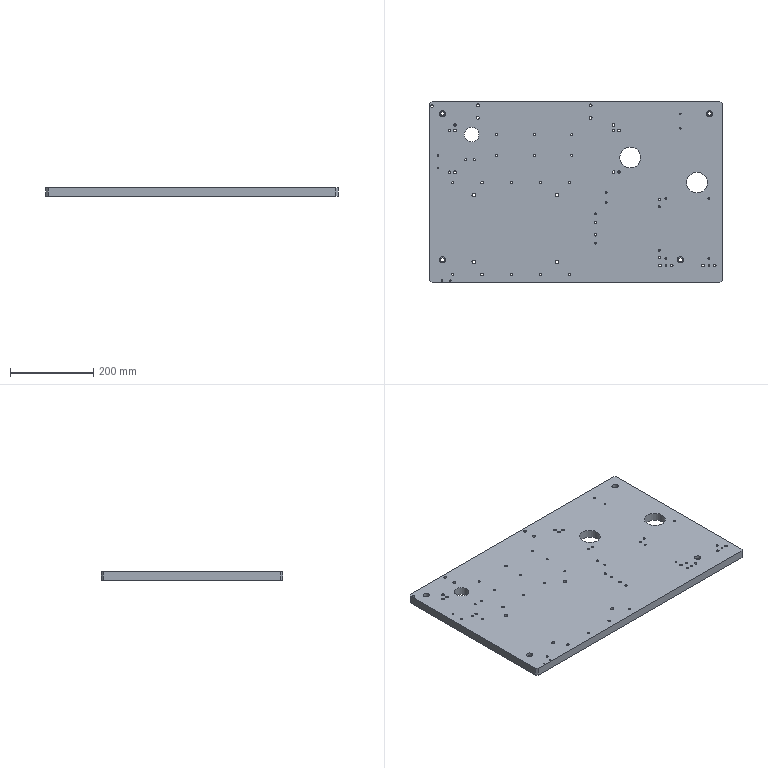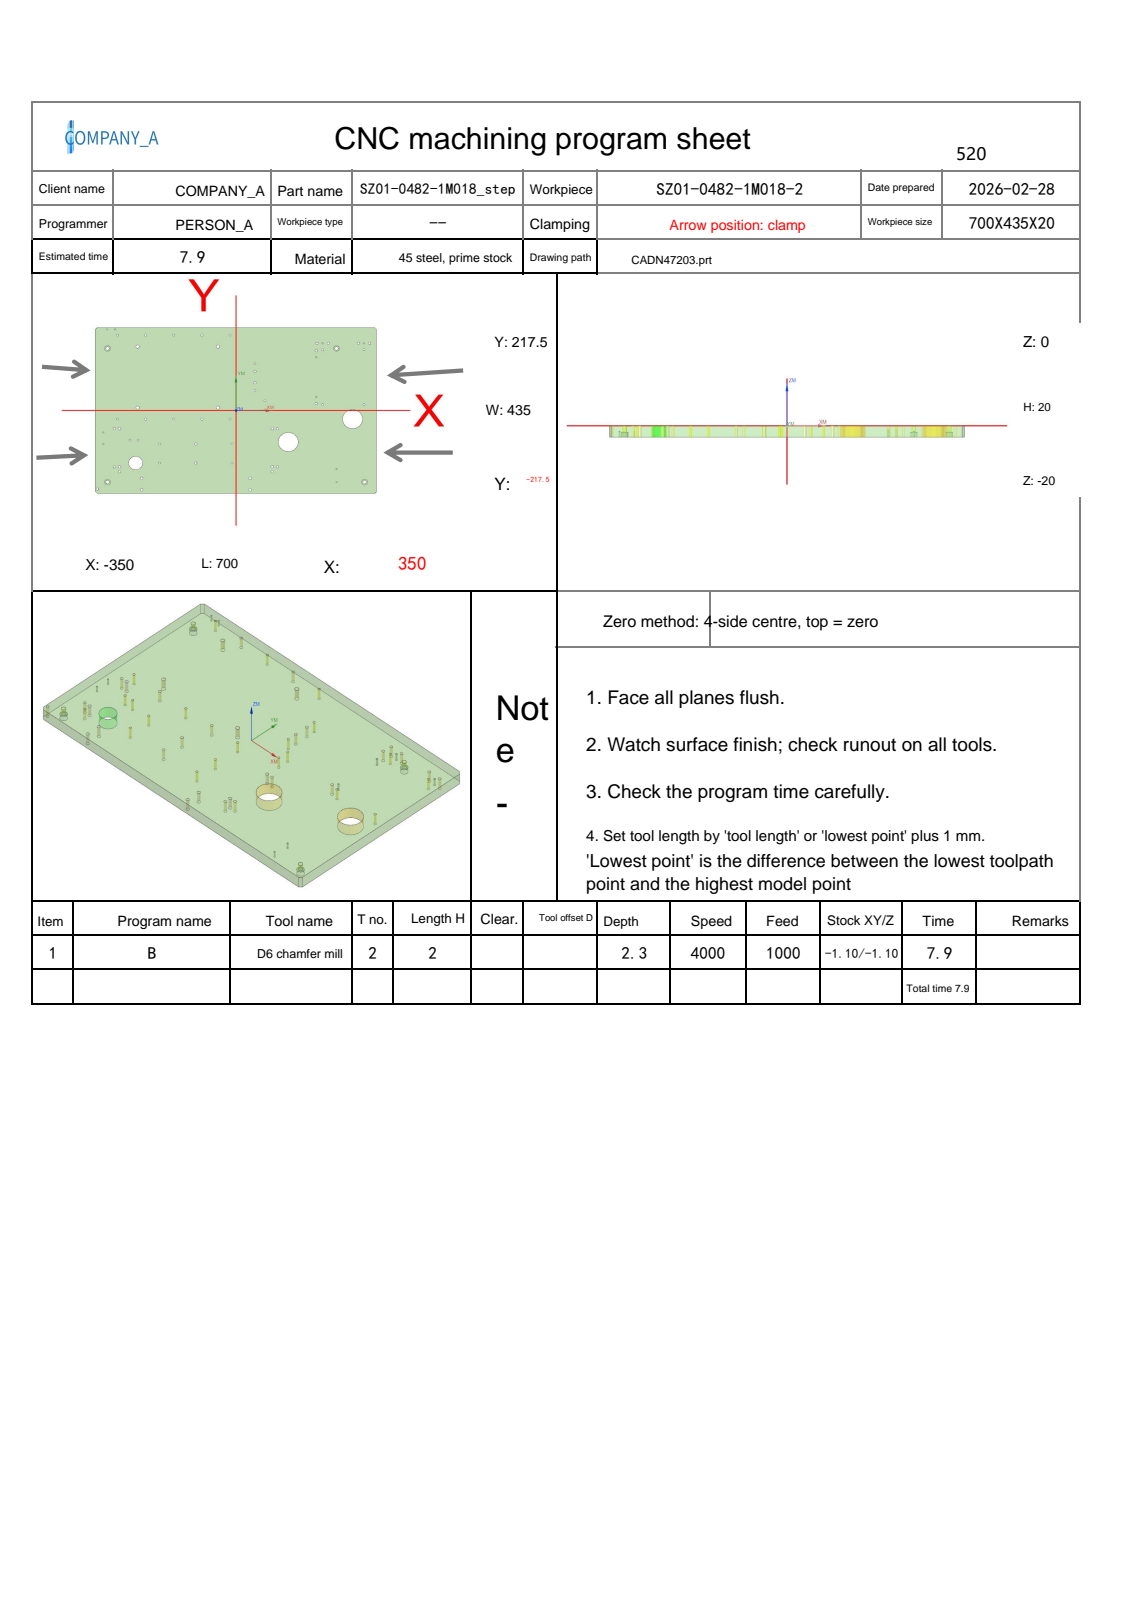NC program | NX | posted by the shop | part box 700 x 435 x 20 mm
Whole program:
%
O0001
(Machine time: 7.52 MIN)
(===Total Tool:1===)
(T2=D6 chamfer mill   D=6.   R=0.   D-  H02 Z=-2.3  )
G80 G90 G17 G49 G40
G91 G28 Z0
M01
N1 T02 M06
(D6 chamfer mill  D=6. R=0. H=02 ce=-0.80 di=-0.80)
G00 G90 G54 X-295.093 Y198.194 M03 S4000
G43 H02 Z50.
M08
Z-1.1
G01 Z-1.6 F300.
X-295.2 Y199.
G03 X-296.7 Y197.5 I0.0 J-1.5
X-295. Y195.8 I1.7 J0.0
X-293.3 Y197.5 I0.0 J1.7
X-295. Y199.2 I-1.7 J0.0
X-296.7 Y197.5 I0.0 J-1.7
X-295.2 Y196. I1.5 J0.0
G01 X-295.093 Y196.806
Z-1.1
G00 Z50.
X-155.093 Y198.194
Z-1.1
G01 Z-1.6
X-155.2 Y199.
G03 X-156.7 Y197.5 I0.0 J-1.5
X-155. Y195.8 I1.7 J0.0
X-153.3 Y197.5 I0.0 J1.7
X-155. Y199.2 I-1.7 J0.0
X-156.7 Y197.5 I0.0 J-1.7
X-155.2 Y196. I1.5 J0.0
G01 X-155.093 Y196.806
Z-1.1
G00 Z50.
X-15.093 Y198.194
Z-1.1
G01 Z-1.6
X-15.2 Y199.
G03 X-16.7 Y197.5 I0.0 J-1.5
X-15. Y195.8 I1.7 J0.0
X-13.3 Y197.5 I0.0 J1.7
X-15. Y199.2 I-1.7 J0.0
X-16.7 Y197.5 I0.0 J-1.7
X-15.2 Y196. I1.5 J0.0
G01 X-15.093 Y196.806
Z-1.1
G00 Z50.
X46.907 Y123.194
Z-1.1
G01 Z-1.6
X46.8 Y124.
G03 X45.3 Y122.5 I0.0 J-1.5
X47. Y120.8 I1.7 J0.0
X48.7 Y122.5 I0.0 J1.7
X47. Y124.2 I-1.7 J0.0
X45.3 Y122.5 I0.0 J-1.7
X46.8 Y121. I1.5 J0.0
G01 X46.907 Y121.806
Z-1.1
G00 Z50.
X215.407 Y160.194
Z-1.1
G01 Z-1.6
X215.3 Y161.
G03 X213.8 Y159.5 I0.0 J-1.5
X215.5 Y157.8 I1.7 J0.0
X217.2 Y159.5 I0.0 J1.7
X215.5 Y161.2 I-1.7 J0.0
X213.8 Y159.5 I0.0 J-1.7
X215.3 Y158. I1.5 J0.0
G01 X215.407 Y158.806
Z-1.1
G00 Z50.
X318.407 Y160.194
Z-1.1
G01 Z-1.6
X318.3 Y161.
G03 X316.8 Y159.5 I0.0 J-1.5
X318.5 Y157.8 I1.7 J0.0
X320.2 Y159.5 I0.0 J1.7
X318.5 Y161.2 I-1.7 J0.0
X316.8 Y159.5 I0.0 J-1.7
X318.3 Y158. I1.5 J0.0
G01 X318.407 Y158.806
Z-1.1
G00 Z50.
Y16.194
Z-1.1
G01 Z-1.6
X318.3 Y17.
G03 X316.8 Y15.5 I0.0 J-1.5
X318.5 Y13.8 I1.7 J0.0
X320.2 Y15.5 I0.0 J1.7
X318.5 Y17.2 I-1.7 J0.0
X316.8 Y15.5 I0.0 J-1.7
X318.3 Y14. I1.5 J0.0
G01 X318.407 Y14.806
Z-1.1
G00 Z50.
X215.407 Y16.194
Z-1.1
G01 Z-1.6
X215.3 Y17.
G03 X213.8 Y15.5 I0.0 J-1.5
X215.5 Y13.8 I1.7 J0.0
X217.2 Y15.5 I0.0 J1.7
X215.5 Y17.2 I-1.7 J0.0
X213.8 Y15.5 I0.0 J-1.7
X215.3 Y14. I1.5 J0.0
G01 X215.407 Y14.806
Z-1.1
G00 Z50.
X71.907 Y2.194
Z-1.1
G01 Z-1.6
X71.8 Y3.
G03 X70.3 Y1.5 I0.0 J-1.5
X72. Y-.2 I1.7 J0.0
X73.7 Y1.5 I0.0 J1.7
X72. Y3.2 I-1.7 J0.0
X70.3 Y1.5 I0.0 J-1.7
X71.8 Y0.0 I1.5 J0.0
G01 X71.907 Y.806
Z-1.1
G00 Z50.
Y26.194
Z-1.1
G01 Z-1.6
X71.8 Y27.
G03 X70.3 Y25.5 I0.0 J-1.5
X72. Y23.8 I1.7 J0.0
X73.7 Y25.5 I0.0 J1.7
X72. Y27.2 I-1.7 J0.0
X70.3 Y25.5 I0.0 J-1.7
X71.8 Y24. I1.5 J0.0
G01 X71.907 Y24.806
Z-1.1
G00 Z50.
X46.907 Y53.194
Z-1.1
G01 Z-1.6
X46.8 Y54.
G03 X45.3 Y52.5 I0.0 J-1.5
X47. Y50.8 I1.7 J0.0
X48.7 Y52.5 I0.0 J1.7
X47. Y54.2 I-1.7 J0.0
X45.3 Y52.5 I0.0 J-1.7
X46.8 Y51. I1.5 J0.0
G01 X46.907 Y51.806
Z-1.1
G00 Z50.
X-15.093 Y-21.806
Z-1.1
G01 Z-1.6
X-15.2 Y-21.
G03 X-16.7 Y-22.5 I0.0 J-1.5
X-15. Y-24.2 I1.7 J0.0
X-13.3 Y-22.5 I0.0 J1.7
X-15. Y-20.8 I-1.7 J0.0
X-16.7 Y-22.5 I0.0 J-1.7
X-15.2 Y-24. I1.5 J0.0
G01 X-15.093 Y-23.194
Z-1.1
G00 Z50.
X-10.093 Y-136.806
Z-1.1
G01 Z-1.6
X-10.2 Y-136.
G03 X-11.7 Y-137.5 I0.0 J-1.5
X-10. Y-139.2 I1.7 J0.0
X-8.3 Y-137.5 I0.0 J1.7
X-10. Y-135.8 I-1.7 J0.0
X-11.7 Y-137.5 I0.0 J-1.7
X-10.2 Y-139. I1.5 J0.0
G01 X-10.093 Y-138.194
Z-1.1
G00 Z50.
Y-86.806
Z-1.1
G01 Z-1.6
X-10.2 Y-86.
G03 X-11.7 Y-87.5 I0.0 J-1.5
X-10. Y-89.2 I1.7 J0.0
X-8.3 Y-87.5 I0.0 J1.7
X-10. Y-85.8 I-1.7 J0.0
X-11.7 Y-87.5 I0.0 J-1.7
X-10.2 Y-89. I1.5 J0.0
G01 X-10.093 Y-88.194
Z-1.1
G00 Z50.
X-155.093 Y-21.806
Z-1.1
G01 Z-1.6
X-155.2 Y-21.
G03 X-156.7 Y-22.5 I0.0 J-1.5
X-155. Y-24.2 I1.7 J0.0
X-153.3 Y-22.5 I0.0 J1.7
X-155. Y-20.8 I-1.7 J0.0
X-156.7 Y-22.5 I0.0 J-1.7
X-155.2 Y-24. I1.5 J0.0
G01 X-155.093 Y-23.194
Z-1.1
G00 Z50.
X-190.093 Y-86.806
Z-1.1
G01 Z-1.6
X-190.2 Y-86.
G03 X-191.7 Y-87.5 I0.0 J-1.5
X-190. Y-89.2 I1.7 J0.0
X-188.3 Y-87.5 I0.0 J1.7
X-190. Y-85.8 I-1.7 J0.0
X-191.7 Y-87.5 I0.0 J-1.7
X-190.2 Y-89. I1.5 J0.0
G01 X-190.093 Y-88.194
Z-1.1
G00 Z50.
Y-136.806
Z-1.1
G01 Z-1.6
X-190.2 Y-136.
G03 X-191.7 Y-137.5 I0.0 J-1.5
X-190. Y-139.2 I1.7 J0.0
X-188.3 Y-137.5 I0.0 J1.7
X-190. Y-135.8 I-1.7 J0.0
X-191.7 Y-137.5 I0.0 J-1.7
X-190.2 Y-139. I1.5 J0.0
G01 X-190.093 Y-138.194
Z-1.1
G00 Z50.
X-244.093 Y-76.806
Z-1.1
G01 Z-1.6
X-244.2 Y-76.
G03 X-245.7 Y-77.5 I0.0 J-1.5
X-244. Y-79.2 I1.7 J0.0
X-242.3 Y-77.5 I0.0 J1.7
X-244. Y-75.8 I-1.7 J0.0
X-245.7 Y-77.5 I0.0 J-1.7
X-244.2 Y-79. I1.5 J0.0
G01 X-244.093 Y-78.194
Z-1.1
G00 Z50.
X-264.093 Y-76.806
Z-1.1
G01 Z-1.6
X-264.2 Y-76.
G03 X-265.7 Y-77.5 I0.0 J-1.5
X-264. Y-79.2 I1.7 J0.0
X-262.3 Y-77.5 I0.0 J1.7
X-264. Y-75.8 I-1.7 J0.0
X-265.7 Y-77.5 I0.0 J-1.7
X-264.2 Y-79. I1.5 J0.0
G01 X-264.093 Y-78.194
Z-1.1
G00 Z50.
X-295.093 Y-21.806
Z-1.1
G01 Z-1.6
X-295.2 Y-21.
G03 X-296.7 Y-22.5 I0.0 J-1.5
X-295. Y-24.2 I1.7 J0.0
X-293.3 Y-22.5 I0.0 J1.7
X-295. Y-20.8 I-1.7 J0.0
X-296.7 Y-22.5 I0.0 J-1.7
X-295.2 Y-24. I1.5 J0.0
G01 X-295.093 Y-23.194
Z-1.1
G00 Z50.
G00 G90 X-225.093 Y198.194 M03 S4000
Z50.
Z-1.1
G01 Z-1.6 F600.
X-225.2 Y199.
G03 X-226.7 Y197.5 I0.0 J-1.5
X-225. Y195.8 I1.7 J0.0
X-223.3 Y197.5 I0.0 J1.7
X-225. Y199.2 I-1.7 J0.0
X-226.7 Y197.5 I0.0 J-1.7
X-225.2 Y196. I1.5 J0.0
G01 X-225.093 Y196.806
Z-1.1
G00 Z50.
X-85.093 Y198.194
Z-1.1
G01 Z-1.6
X-85.2 Y199.
G03 X-86.7 Y197.5 I0.0 J-1.5
X-85. Y195.8 I1.7 J0.0
X-83.3 Y197.5 I0.0 J1.7
X-85. Y199.2 I-1.7 J0.0
X-86.7 Y197.5 I0.0 J-1.7
X-85.2 Y196. I1.5 J0.0
G01 X-85.093 Y196.806
Z-1.1
G00 Z50.
X46.907 Y103.194
Z-1.1
G01 Z-1.6
X46.8 Y104.
G03 X45.3 Y102.5 I0.0 J-1.5
X47. Y100.8 I1.7 J0.0
X48.7 Y102.5 I0.0 J1.7
X47. Y104.2 I-1.7 J0.0
X45.3 Y102.5 I0.0 J-1.7
X46.8 Y101. I1.5 J0.0
G01 X46.907 Y101.806
Z-1.1
G00 Z50.
Y73.194
Z-1.1
G01 Z-1.6
X46.8 Y74.
G03 X45.3 Y72.5 I0.0 J-1.5
X47. Y70.8 I1.7 J0.0
X48.7 Y72.5 I0.0 J1.7
X47. Y74.2 I-1.7 J0.0
X45.3 Y72.5 I0.0 J-1.7
X46.8 Y71. I1.5 J0.0
G01 X46.907 Y71.806
Z-1.1
G00 Z50.
X201.407 Y176.694
Z-1.1
G01 Z-1.6
X201.3 Y177.5
G03 X199.8 Y176. I0.0 J-1.5
X201.5 Y174.3 I1.7 J0.0
X203.2 Y176. I0.0 J1.7
X201.5 Y177.7 I-1.7 J0.0
X199.8 Y176. I0.0 J-1.7
X201.3 Y174.5 I1.5 J0.0
G01 X201.407 Y175.306
Z-1.1
G00 Z50.
X304.407 Y176.694
Z-1.1
G01 Z-1.6
X304.3 Y177.5
G03 X302.8 Y176. I0.0 J-1.5
X304.5 Y174.3 I1.7 J0.0
X306.2 Y176. I0.0 J1.7
X304.5 Y177.7 I-1.7 J0.0
X302.8 Y176. I0.0 J-1.7
X304.3 Y174.5 I1.5 J0.0
G01 X304.407 Y175.306
Z-1.1
G00 Z50.
X332.407 Y176.694
Z-1.1
G01 Z-1.6
X332.3 Y177.5
G03 X330.8 Y176. I0.0 J-1.5
X332.5 Y174.3 I1.7 J0.0
X334.2 Y176. I0.0 J1.7
X332.5 Y177.7 I-1.7 J0.0
X330.8 Y176. I0.0 J-1.7
X332.3 Y174.5 I1.5 J0.0
G01 X332.407 Y175.306
Z-1.1
G00 Z50.
X229.407 Y176.694
Z-1.1
G01 Z-1.6
X229.3 Y177.5
G03 X227.8 Y176. I0.0 J-1.5
X229.5 Y174.3 I1.7 J0.0
X231.2 Y176. I0.0 J1.7
X229.5 Y177.7 I-1.7 J0.0
X227.8 Y176. I0.0 J-1.7
X229.3 Y174.5 I1.5 J0.0
G01 X229.407 Y175.306
Z-1.1
G00 Z50.
X199.407 Y157.194
Z-1.1
G01 Z-1.6
X199.3 Y158.
G03 X197.8 Y156.5 I0.0 J-1.5
X199.5 Y154.8 I1.7 J0.0
X201.2 Y156.5 I0.0 J1.7
X199.5 Y158.2 I-1.7 J0.0
X197.8 Y156.5 I0.0 J-1.7
X199.3 Y155. I1.5 J0.0
G01 X199.407 Y155.806
Z-1.1
G00 Z50.
Y19.194
Z-1.1
G01 Z-1.6
X199.3 Y20.
G03 X197.8 Y18.5 I0.0 J-1.5
X199.5 Y16.8 I1.7 J0.0
X201.2 Y18.5 I0.0 J1.7
X199.5 Y20.2 I-1.7 J0.0
X197.8 Y18.5 I0.0 J-1.7
X199.3 Y17. I1.5 J0.0
G01 X199.407 Y17.806
Z-1.1
G00 Z50.
X102.907 Y-46.806
Z-1.1
G01 Z-1.6
X102.8 Y-46.
G03 X101.3 Y-47.5 I0.0 J-1.5
X103. Y-49.2 I1.7 J0.0
X104.7 Y-47.5 I0.0 J1.7
X103. Y-45.8 I-1.7 J0.0
X101.3 Y-47.5 I0.0 J-1.7
X102.8 Y-49. I1.5 J0.0
G01 X102.907 Y-48.194
Z-1.1
G00 Z50.
Y-146.806
Z-1.1
G01 Z-1.6
X102.8 Y-146.
G03 X101.3 Y-147.5 I0.0 J-1.5
X103. Y-149.2 I1.7 J0.0
X104.7 Y-147.5 I0.0 J1.7
X103. Y-145.8 I-1.7 J0.0
X101.3 Y-147.5 I0.0 J-1.7
X102.8 Y-149. I1.5 J0.0
G01 X102.907 Y-148.194
Z-1.1
G00 Z50.
X89.907 Y-159.806
Z-1.1
G01 Z-1.6
X89.8 Y-159.
G03 X88.3 Y-160.5 I0.0 J-1.5
X90. Y-162.2 I1.7 J0.0
X91.7 Y-160.5 I0.0 J1.7
X90. Y-158.8 I-1.7 J0.0
X88.3 Y-160.5 I0.0 J-1.7
X89.8 Y-162. I1.5 J0.0
G01 X89.907 Y-161.194
Z-1.1
G00 Z50.
X-100.093 Y-136.806
Z-1.1
G01 Z-1.6
X-100.2 Y-136.
G03 X-101.7 Y-137.5 I0.0 J-1.5
X-100. Y-139.2 I1.7 J0.0
X-98.3 Y-137.5 I0.0 J1.7
X-100. Y-135.8 I-1.7 J0.0
X-101.7 Y-137.5 I0.0 J-1.7
X-100.2 Y-139. I1.5 J0.0
G01 X-100.093 Y-138.194
Z-1.1
G00 Z50.
Y-86.806
Z-1.1
G01 Z-1.6
X-100.2 Y-86.
G03 X-101.7 Y-87.5 I0.0 J-1.5
X-100. Y-89.2 I1.7 J0.0
X-98.3 Y-87.5 I0.0 J1.7
X-100. Y-85.8 I-1.7 J0.0
X-101.7 Y-87.5 I0.0 J-1.7
X-100.2 Y-89. I1.5 J0.0
G01 X-100.093 Y-88.194
Z-1.1
G00 Z50.
X-85.093 Y-21.806
Z-1.1
G01 Z-1.6
X-85.2 Y-21.
G03 X-86.7 Y-22.5 I0.0 J-1.5
X-85. Y-24.2 I1.7 J0.0
X-83.3 Y-22.5 I0.0 J1.7
X-85. Y-20.8 I-1.7 J0.0
X-86.7 Y-22.5 I0.0 J-1.7
X-85.2 Y-24. I1.5 J0.0
G01 X-85.093 Y-23.194
Z-1.1
G00 Z50.
X-225.093 Y-21.806
Z-1.1
G01 Z-1.6
X-225.2 Y-21.
G03 X-226.7 Y-22.5 I0.0 J-1.5
X-225. Y-24.2 I1.7 J0.0
X-223.3 Y-22.5 I0.0 J1.7
X-225. Y-20.8 I-1.7 J0.0
X-226.7 Y-22.5 I0.0 J-1.7
X-225.2 Y-24. I1.5 J0.0
G01 X-225.093 Y-23.194
Z-1.1
G00 Z50.
X-303.093 Y-46.806
Z-1.1
G01 Z-1.6
X-303.2 Y-46.
G03 X-304.7 Y-47.5 I0.0 J-1.5
X-303. Y-49.2 I1.7 J0.0
X-301.3 Y-47.5 I0.0 J1.7
X-303. Y-45.8 I-1.7 J0.0
X-304.7 Y-47.5 I0.0 J-1.7
X-303.2 Y-49. I1.5 J0.0
G01 X-303.093 Y-48.194
Z-1.1
G00 Z50.
Y-146.806
Z-1.1
G01 Z-1.6
X-303.2 Y-146.
G03 X-304.7 Y-147.5 I0.0 J-1.5
X-303. Y-149.2 I1.7 J0.0
X-301.3 Y-147.5 I0.0 J1.7
X-303. Y-145.8 I-1.7 J0.0
X-304.7 Y-147.5 I0.0 J-1.7
X-303.2 Y-149. I1.5 J0.0
G01 X-303.093 Y-148.194
Z-1.1
G00 Z50.
X-290.093 Y-159.806
Z-1.1
G01 Z-1.6
X-290.2 Y-159.
G03 X-291.7 Y-160.5 I0.0 J-1.5
X-290. Y-162.2 I1.7 J0.0
X-288.3 Y-160.5 I0.0 J1.7
X-290. Y-158.8 I-1.7 J0.0
X-291.7 Y-160.5 I0.0 J-1.7
X-290.2 Y-162. I1.5 J0.0
G01 X-290.093 Y-161.194
Z-1.1
G00 Z50.
X-345.093 Y-204.806
Z-1.1
G01 Z-1.6
X-345.2 Y-204.
G03 X-346.7 Y-205.5 I0.0 J-1.5
X-345. Y-207.2 I1.7 J0.0
X-343.3 Y-205.5 I0.0 J1.7
X-345. Y-203.8 I-1.7 J0.0
X-346.7 Y-205.5 I0.0 J-1.7
X-345.2 Y-207. I1.5 J0.0
G01 X-345.093 Y-206.194
Z-1.1
G00 Z50.
G00 G90 X-290.995 Y-46. M03 S4000
Z50.
Z-1.1
G01 Z-1.6 F300.
X-291.3
G03 X-292.8 Y-47.5 I0.0 J-1.5
X-290. Y-50.3 I2.8 J0.0
X-287.2 Y-47.5 I0.0 J2.8
X-290. Y-44.7 I-2.8 J0.0
X-292.8 Y-47.5 I0.0 J-2.8
X-291.3 Y-49. I1.5 J0.0
G01 X-290.995
Z-1.1
G00 Z50.
Y-146.
Z-1.1
G01 Z-1.6
X-291.3
G03 X-292.8 Y-147.5 I0.0 J-1.5
X-290. Y-150.3 I2.8 J0.0
X-287.2 Y-147.5 I0.0 J2.8
X-290. Y-144.7 I-2.8 J0.0
X-292.8 Y-147.5 I0.0 J-2.8
X-291.3 Y-149. I1.5 J0.0
G01 X-290.995
Z-1.1
G00 Z50.
X-235.995 Y-176.
Z-1.1
G01 Z-1.6
X-236.3
G03 X-237.8 Y-177.5 I0.0 J-1.5
X-235. Y-180.3 I2.8 J0.0
X-232.2 Y-177.5 I0.0 J2.8
X-235. Y-174.7 I-2.8 J0.0
X-237.8 Y-177.5 I0.0 J-2.8
X-236.3 Y-179. I1.5 J0.0
G01 X-235.995
Z-1.1
G00 Z50.
Y-206.
Z-1.1
G01 Z-1.6
X-236.3
G03 X-237.8 Y-207.5 I0.0 J-1.5
X-235. Y-210.3 I2.8 J0.0
X-232.2 Y-207.5 I0.0 J2.8
X-235. Y-204.7 I-2.8 J0.0
X-237.8 Y-207.5 I0.0 J-2.8
X-236.3 Y-209. I1.5 J0.0
G01 X-235.995
Z-1.1
G00 Z50.
X34.005 Y-206.
Z-1.1
G01 Z-1.6
X33.7
G03 X32.2 Y-207.5 I0.0 J-1.5
X35. Y-210.3 I2.8 J0.0
X37.8 Y-207.5 I0.0 J2.8
X35. Y-204.7 I-2.8 J0.0
X32.2 Y-207.5 I0.0 J-2.8
X33.7 Y-209. I1.5 J0.0
G01 X34.005
Z-1.1
G00 Z50.
Y-176.
Z-1.1
G01 Z-1.6
X33.7
G03 X32.2 Y-177.5 I0.0 J-1.5
X35. Y-180.3 I2.8 J0.0
X37.8 Y-177.5 I0.0 J2.8
X35. Y-174.7 I-2.8 J0.0
X32.2 Y-177.5 I0.0 J-2.8
X33.7 Y-179. I1.5 J0.0
G01 X34.005
Z-1.1
G00 Z50.
X89.005 Y-146.
Z-1.1
G01 Z-1.6
X88.7
G03 X87.2 Y-147.5 I0.0 J-1.5
X90. Y-150.3 I2.8 J0.0
X92.8 Y-147.5 I0.0 J2.8
X90. Y-144.7 I-2.8 J0.0
X87.2 Y-147.5 I0.0 J-2.8
X88.7 Y-149. I1.5 J0.0
G01 X89.005
Z-1.1
G00 Z50.
Y-46.
Z-1.1
G01 Z-1.6
X88.7
G03 X87.2 Y-47.5 I0.0 J-1.5
X90. Y-50.3 I2.8 J0.0
X92.8 Y-47.5 I0.0 J2.8
X90. Y-44.7 I-2.8 J0.0
X87.2 Y-47.5 I0.0 J-2.8
X88.7 Y-49. I1.5 J0.0
G01 X89.005
Z-1.1
G00 Z50.
G00 G90 X-45.777 Y10.242 M03 S3000
Z50.
Z-1.
G01 Z-1.5 F400.
X-45.85 Y10.5
G03 X-48.85 Y7.5 I0.0 J-3.
X-45. Y3.65 I3.85 J0.0
X-41.15 Y7.5 I0.0 J3.85
X-45. Y11.35 I-3.85 J0.0
X-48.85 Y7.5 I0.0 J-3.85
X-45.85 Y4.5 I3. J0.0
G01 X-45.777 Y4.758
Z-1.
G00 Z50.
Y170.242
Z-1.
G01 Z-1.5
X-45.85 Y170.5
G03 X-48.85 Y167.5 I0.0 J-3.
X-45. Y163.65 I3.85 J0.0
X-41.15 Y167.5 I0.0 J3.85
X-45. Y171.35 I-3.85 J0.0
X-48.85 Y167.5 I0.0 J-3.85
X-45.85 Y164.5 I3. J0.0
G01 X-45.777 Y164.758
Z-1.
G00 Z50.
X-245.777 Y170.242
Z-1.
G01 Z-1.5
X-245.85 Y170.5
G03 X-248.85 Y167.5 I0.0 J-3.
X-245. Y163.65 I3.85 J0.0
X-241.15 Y167.5 I0.0 J3.85
X-245. Y171.35 I-3.85 J0.0
X-248.85 Y167.5 I0.0 J-3.85
X-245.85 Y164.5 I3. J0.0
G01 X-245.777 Y164.758
Z-1.
G00 Z50.
Y10.242
Z-1.
G01 Z-1.5
X-245.85 Y10.5
G03 X-248.85 Y7.5 I0.0 J-3.
X-245. Y3.65 I3.85 J0.0
X-241.15 Y7.5 I0.0 J3.85
X-245. Y11.35 I-3.85 J0.0
X-248.85 Y7.5 I0.0 J-3.85
X-245.85 Y4.5 I3. J0.0
G01 X-245.777 Y4.758
Z-1.
G00 Z50.
G00 G90 X-320.001 Y-186. M03 S3000
Z50.
Z-1.8
G01 Z-2.3 F600.
X-321.
G03 X-322.5 Y-187.5 I0.0 J-1.5
X-320. Y-190. I2.5 J0.0
X-317.5 Y-187.5 I0.0 J2.5
X-320. Y-185. I-2.5 J0.0
X-322.5 Y-187.5 I0.0 J-2.5
X-321. Y-189. I1.5 J0.0
G01 X-320.001
Z-1.8
G00 Z50.
Y164.
Z-1.8
G01 Z-2.3
X-321.
G03 X-322.5 Y162.5 I0.0 J-1.5
X-320. Y160. I2.5 J0.0
X-317.5 Y162.5 I0.0 J2.5
X-320. Y165. I-2.5 J0.0
X-322.5 Y162.5 I0.0 J-2.5
X-321. Y161. I1.5 J0.0
G01 X-320.001
Z-1.8
G00 Z50.
X249.999 Y164.
Z-1.8
G01 Z-2.3
X249.
G03 X247.5 Y162.5 I0.0 J-1.5
X250. Y160. I2.5 J0.0
X252.5 Y162.5 I0.0 J2.5
X250. Y165. I-2.5 J0.0
X247.5 Y162.5 I0.0 J-2.5
X249. Y161. I1.5 J0.0
G01 X250.
Z-1.8
G00 Z50.
X319.999 Y-186.
Z-1.8
G01 Z-2.3
X319.
G03 X317.5 Y-187.5 I0.0 J-1.5
X320. Y-190. I2.5 J0.0
X322.5 Y-187.5 I0.0 J2.5
X320. Y-185. I-2.5 J0.0
X317.5 Y-187.5 I0.0 J-2.5
X319. Y-189. I1.5 J0.0
G01 X319.999
Z-1.8
G00 Z50.
G00 G90 X-351.375 Y212.257 M03 S3500
Z47.5
Z.055
G01 Z-1.2 F1000.
G03 X-351.069 Y212.423 I-.795 J1.835
G01 X-351.022 Y212.45
X-351. Y212.5
X-350.966 Y212.759
X-350.866 Y213.
X-350.707 Y213.207
X-345.707 Y218.207
X-345.5 Y218.366
X-345.259 Y218.466
X-345. Y218.5
X345.
X345.259 Y218.466
X345.5 Y218.366
X345.707 Y218.207
X350.707 Y213.207
X350.744 Y213.167
X350.797 Y213.155
G03 X351.14 Y213.095 I.518 J1.932
G01 Z.113
G00 Z47.5
Y-213.095
Z.113
G01 Z-1.2
G03 X350.797 Y-213.155 I.174 J-1.992
G01 X350.744 Y-213.167
X350.707 Y-213.207
X345.707 Y-218.207
X345.5 Y-218.366
X345.259 Y-218.466
X345. Y-218.5
X-345.
X-345.259 Y-218.466
X-345.5 Y-218.366
X-345.707 Y-218.207
X-350.707 Y-213.207
X-350.744 Y-213.167
X-350.797 Y-213.155
G03 X-351.14 Y-213.095 I-.518 J-1.932
G01 Z.113
G00 Z2.55
X-346.808 Y-205.096
Z.257
G01 Z-1.2
G03 X-346.982 Y-205.398 I1.638 J-1.147
G01 X-347.008 Y-205.446
X-347. Y-205.5
G03 X-345. Y-207.5 I2. J0.0
X-343. Y-205.5 I0.0 J2.
X-345. Y-203.5 I-2. J0.0
X-346.97 Y-205.153 I0.0 J-2.
G01 X-347. Y-205.5
X-347.008 Y-205.554
X-346.982 Y-205.602
G03 X-346.808 Y-205.904 I1.813 J.845
G01 Z.257
G00 Z47.5
X-323.303 Y-187.099
Z.23
G01 Z-1.2
G03 X-323.481 Y-187.398 I1.624 J-1.167
G01 X-323.507 Y-187.446
X-323.5 Y-187.5
G03 X-320. Y-191. I3.5 J0.0
X-316.5 Y-187.5 I0.0 J3.5
X-320. Y-184. I-3.5 J0.0
X-323.5 Y-187.5 I0.0 J-3.5
G01 X-323.507 Y-187.554
X-323.481 Y-187.602
G03 X-323.303 Y-187.901 I1.802 J.868
G01 Z.23
G00 Z47.5
X-291.808 Y-160.096
Z.257
G01 Z-1.2
G03 X-291.982 Y-160.398 I1.638 J-1.147
G01 X-292.008 Y-160.446
X-292. Y-160.5
G03 X-290. Y-162.5 I2. J0.0
X-288. Y-160.5 I0.0 J2.
X-290. Y-158.5 I-2. J0.0
X-291.97 Y-160.153 I0.0 J-2.
G01 X-292. Y-160.5
X-292.008 Y-160.554
X-291.982 Y-160.602
G03 X-291.808 Y-160.904 I1.813 J.845
G01 Z.257
G00 Z47.5
X-304.808 Y-147.096
Z.257
G01 Z-1.2
G03 X-304.982 Y-147.398 I1.638 J-1.147
G01 X-305.008 Y-147.446
X-305. Y-147.5
G03 X-303. Y-149.5 I2. J0.0
X-301. Y-147.5 I0.0 J2.
X-303. Y-145.5 I-2. J0.0
X-304.97 Y-147.153 I0.0 J-2.
G01 X-305. Y-147.5
X-305.008 Y-147.554
X-304.982 Y-147.602
G03 X-304.808 Y-147.904 I1.813 J.845
G01 Z.257
G00 Z47.5
X-292.208 Y-147.096
Z.252
G01 Z-1.2
G03 X-292.382 Y-147.398 I1.638 J-1.147
G01 X-292.408 Y-147.446
X-292.4 Y-147.5
G03 X-290. Y-149.9 I2.4 J0.0
X-287.6 Y-147.5 I0.0 J2.4
X-290. Y-145.1 I-2.4 J0.0
X-292.4 Y-147.5 I0.0 J-2.4
G01 X-292.408 Y-147.554
X-292.382 Y-147.602
G03 X-292.208 Y-147.904 I1.813 J.845
G01 Z.252
G00 Z47.5
X-266.286 Y-137.107
Z.195
G01 Z-1.2
G03 X-266.476 Y-137.399 I1.573 J-1.235
G01 X-266.505 Y-137.446
X-266.5 Y-137.5
G03 X-250. Y-154. I16.5 J0.0
X-233.5 Y-137.5 I0.0 J16.5
X-250. Y-121. I-16.5 J0.0
X-266.5 Y-137.5 I0.0 J-16.5
G01 X-266.505 Y-137.554
X-266.476 Y-137.601
G03 X-266.286 Y-137.893 I1.764 J.943
G01 Z.195
G00 Z47.5
X-237.208 Y-177.096
Z.252
G01 Z-1.2
G03 X-237.382 Y-177.398 I1.638 J-1.147
G01 X-237.408 Y-177.446
X-237.4 Y-177.5
G03 X-235. Y-179.9 I2.4 J0.0
X-232.6 Y-177.5 I0.0 J2.4
X-235. Y-175.1 I-2.4 J0.0
X-237.4 Y-177.5 I0.0 J-2.4
G01 X-237.408 Y-177.554
X-237.382 Y-177.602
G03 X-237.208 Y-177.904 I1.813 J.845
G01 Z.252
G00 Z47.5
Y-207.096
Z.252
G01 Z-1.2
G03 X-237.382 Y-207.398 I1.638 J-1.147
G01 X-237.408 Y-207.446
X-237.4 Y-207.5
G03 X-235. Y-209.9 I2.4 J0.0
X-232.6 Y-207.5 I0.0 J2.4
X-235. Y-205.1 I-2.4 J0.0
X-237.4 Y-207.5 I0.0 J-2.4
G01 X-237.408 Y-207.554
X-237.382 Y-207.602
G03 X-237.208 Y-207.904 I1.813 J.845
G01 Z.252
G00 Z47.5
X-191.315 Y-137.093
Z.284
G01 Z-1.2
G03 X-191.484 Y-137.398 I1.658 J-1.118
G01 X-191.509 Y-137.446
X-191.5 Y-137.5
G03 X-190. Y-139. I1.5 J0.0
X-188.5 Y-137.5 I0.0 J1.5
X-190. Y-136. I-1.5 J0.0
X-191.5 Y-137.5 I0.0 J-1.5
G01 X-191.509 Y-137.554
X-191.484 Y-137.602
G03 X-191.315 Y-137.907 I1.827 J.813
G01 Z.284
G00 Z47.5
Y-87.093
Z.284
G01 Z-1.2
G03 X-191.484 Y-87.398 I1.658 J-1.118
G01 X-191.509 Y-87.446
X-191.5 Y-87.5
G03 X-190. Y-89. I1.5 J0.0
X-188.5 Y-87.5 I0.0 J1.5
X-190. Y-86. I-1.5 J0.0
X-191.5 Y-87.5 I0.0 J-1.5
G01 X-191.509 Y-87.554
X-191.484 Y-87.602
G03 X-191.315 Y-87.907 I1.827 J.813
G01 Z.284
G00 Z47.5
X-245.315 Y-77.093
Z.284
G01 Z-1.2
G03 X-245.484 Y-77.398 I1.658 J-1.118
G01 X-245.509 Y-77.446
X-245.5 Y-77.5
G03 X-244. Y-79. I1.5 J0.0
X-242.5 Y-77.5 I0.0 J1.5
X-244. Y-76. I-1.5 J0.0
X-245.5 Y-77.5 I0.0 J-1.5
G01 X-245.509 Y-77.554
X-245.484 Y-77.602
G03 X-245.315 Y-77.907 I1.827 J.813
G01 Z.284
G00 Z47.5
X-265.315 Y-77.093
Z.284
G01 Z-1.2
G03 X-265.484 Y-77.398 I1.658 J-1.118
G01 X-265.509 Y-77.446
X-265.5 Y-77.5
G03 X-264. Y-79. I1.5 J0.0
X-262.5 Y-77.5 I0.0 J1.5
X-264. Y-76. I-1.5 J0.0
X-265.5 Y-77.5 I0.0 J-1.5
G01 X-265.509 Y-77.554
X-265.484 Y-77.602
G03 X-265.315 Y-77.907 I1.827 J.813
G01 Z.284
G00 Z47.5
X-292.208 Y-47.096
Z.252
G01 Z-1.2
G03 X-292.382 Y-47.398 I1.638 J-1.147
G01 X-292.408 Y-47.446
X-292.4 Y-47.5
G03 X-290. Y-49.9 I2.4 J0.0
X-287.6 Y-47.5 I0.0 J2.4
X-290. Y-45.1 I-2.4 J0.0
X-292.4 Y-47.5 I0.0 J-2.4
G01 X-292.408 Y-47.554
X-292.382 Y-47.602
G03 X-292.208 Y-47.904 I1.813 J.845
G01 Z.252
G00 Z47.5
X-304.808 Y-47.096
Z.257
G01 Z-1.2
G03 X-304.982 Y-47.398 I1.638 J-1.147
G01 X-305.008 Y-47.446
X-305. Y-47.5
G03 X-303. Y-49.5 I2. J0.0
X-301. Y-47.5 I0.0 J2.
X-303. Y-45.5 I-2. J0.0
X-304.97 Y-47.153 I0.0 J-2.
G01 X-305. Y-47.5
X-305.008 Y-47.554
X-304.982 Y-47.602
G03 X-304.808 Y-47.904 I1.813 J.845
G01 Z.257
G00 Z47.5
X-296.315 Y-22.093
Z.284
G01 Z-1.2
G03 X-296.484 Y-22.398 I1.658 J-1.118
G01 X-296.509 Y-22.446
X-296.5 Y-22.5
G03 X-295. Y-24. I1.5 J0.0
X-293.5 Y-22.5 I0.0 J1.5
X-295. Y-21. I-1.5 J0.0
X-296.5 Y-22.5 I0.0 J-1.5
G01 X-296.509 Y-22.554
X-296.484 Y-22.602
G03 X-296.315 Y-22.907 I1.827 J.813
G01 Z.284
G00 Z47.5
X-226.808 Y-22.096
Z.257
G01 Z-1.2
G03 X-226.982 Y-22.398 I1.638 J-1.147
G01 X-227.008 Y-22.446
X-227. Y-22.5
G03 X-225. Y-24.5 I2. J0.0
X-223. Y-22.5 I0.0 J2.
X-225. Y-20.5 I-2. J0.0
X-226.97 Y-22.153 I0.0 J-2.
G01 X-227. Y-22.5
X-227.008 Y-22.554
X-226.982 Y-22.602
G03 X-226.808 Y-22.904 I1.813 J.845
G01 Z.257
G00 Z47.5
X-248.053 Y7.901
Z.232
G01 Z-1.2
G03 X-248.231 Y7.602 I1.624 J-1.167
G01 X-248.257 Y7.554
X-248.25 Y7.5
G03 X-245. Y4.25 I3.25 J0.0
X-241.75 Y7.5 I0.0 J3.25
X-245. Y10.75 I-3.25 J0.0
X-248.25 Y7.5 I0.0 J-3.25
G01 X-248.257 Y7.446
X-248.231 Y7.398
G03 X-248.053 Y7.099 I1.802 J.868
G01 Z.232
G00 Z47.5
X-323.303 Y162.901
Z.23
G01 Z-1.2
G03 X-323.481 Y162.602 I1.624 J-1.167
G01 X-323.507 Y162.554
X-323.5 Y162.5
G03 X-320. Y159. I3.5 J0.0
X-316.5 Y162.5 I0.0 J3.5
X-320. Y166. I-3.5 J0.0
X-323.5 Y162.5 I0.0 J-3.5
G01 X-323.507 Y162.446
X-323.481 Y162.398
G03 X-323.303 Y162.099 I1.802 J.868
G01 Z.23
G00 Z47.5
X-296.315 Y197.907
Z.284
G01 Z-1.2
G03 X-296.484 Y197.602 I1.658 J-1.118
G01 X-296.509 Y197.554
X-296.5 Y197.5
G03 X-295. Y196. I1.5 J0.0
X-293.5 Y197.5 I0.0 J1.5
X-295. Y199. I-1.5 J0.0
X-296.5 Y197.5 I0.0 J-1.5
G01 X-296.509 Y197.446
X-296.484 Y197.398
G03 X-296.315 Y197.093 I1.827 J.813
G01 Z.284
G00 Z47.5
X-248.053 Y167.901
Z.232
G01 Z-1.2
G03 X-248.231 Y167.602 I1.624 J-1.167
G01 X-248.257 Y167.554
X-248.25 Y167.5
G03 X-245. Y164.25 I3.25 J0.0
X-241.75 Y167.5 I0.0 J3.25
X-245. Y170.75 I-3.25 J0.0
X-248.25 Y167.5 I0.0 J-3.25
G01 X-248.257 Y167.446
X-248.231 Y167.398
G03 X-248.053 Y167.099 I1.802 J.868
G01 Z.232
G00 Z47.5
X-226.808 Y197.904
Z.257
G01 Z-1.2
G03 X-226.982 Y197.602 I1.638 J-1.147
G01 X-227.008 Y197.554
X-227. Y197.5
G03 X-225. Y195.5 I2. J0.0
X-223. Y197.5 I0.0 J2.
X-225. Y199.5 I-2. J0.0
X-226.97 Y197.847 I0.0 J-2.
G01 X-227. Y197.5
X-227.008 Y197.446
X-226.982 Y197.398
G03 X-226.808 Y197.096 I1.813 J.845
G01 Z.257
G00 Z47.5
X-156.315 Y197.907
Z.284
G01 Z-1.2
G03 X-156.484 Y197.602 I1.658 J-1.118
G01 X-156.509 Y197.554
X-156.5 Y197.5
G03 X-155. Y196. I1.5 J0.0
X-153.5 Y197.5 I0.0 J1.5
X-155. Y199. I-1.5 J0.0
X-156.5 Y197.5 I0.0 J-1.5
G01 X-156.509 Y197.446
X-156.484 Y197.398
G03 X-156.315 Y197.093 I1.827 J.813
G01 Z.284
G00 Z47.5
X-86.808 Y197.904
Z.257
G01 Z-1.2
G03 X-86.982 Y197.602 I1.638 J-1.147
G01 X-87.008 Y197.554
X-87. Y197.5
G03 X-85. Y195.5 I2. J0.0
X-83. Y197.5 I0.0 J2.
X-85. Y199.5 I-2. J0.0
X-86.97 Y197.847 I0.0 J-2.
G01 X-87. Y197.5
X-87.008 Y197.446
X-86.982 Y197.398
G03 X-86.808 Y197.096 I1.813 J.845
G01 Z.257
G00 Z47.5
X-48.053 Y167.901
Z.232
G01 Z-1.2
G03 X-48.231 Y167.602 I1.624 J-1.167
G01 X-48.257 Y167.554
X-48.25 Y167.5
G03 X-45. Y164.25 I3.25 J0.0
X-41.75 Y167.5 I0.0 J3.25
X-45. Y170.75 I-3.25 J0.0
X-48.25 Y167.5 I0.0 J-3.25
G01 X-48.257 Y167.446
X-48.231 Y167.398
G03 X-48.053 Y167.099 I1.802 J.868
G01 Z.232
G00 Z47.5
X-16.315 Y197.907
Z.284
G01 Z-1.2
G03 X-16.484 Y197.602 I1.658 J-1.118
G01 X-16.509 Y197.554
X-16.5 Y197.5
G03 X-15. Y196. I1.5 J0.0
X-13.5 Y197.5 I0.0 J1.5
X-15. Y199. I-1.5 J0.0
X-16.5 Y197.5 I0.0 J-1.5
G01 X-16.509 Y197.446
X-16.484 Y197.398
G03 X-16.315 Y197.093 I1.827 J.813
G01 Z.284
G00 Z47.5
X45.685 Y122.907
Z.284
G01 Z-1.2
G03 X45.516 Y122.602 I1.658 J-1.118
G01 X45.491 Y122.554
X45.5 Y122.5
G03 X47. Y121. I1.5 J0.0
X48.5 Y122.5 I0.0 J1.5
X47. Y124. I-1.5 J0.0
X45.5 Y122.5 I0.0 J-1.5
G01 X45.491 Y122.446
X45.516 Y122.398
G03 X45.685 Y122.093 I1.827 J.813
G01 Z.284
G00 Z47.5
X45.192 Y102.904
Z.257
G01 Z-1.2
G03 X45.018 Y102.602 I1.638 J-1.147
G01 X44.992 Y102.554
X45. Y102.5
G03 X47. Y100.5 I2. J0.0
X49. Y102.5 I0.0 J2.
X47. Y104.5 I-2. J0.0
X45.03 Y102.847 I0.0 J-2.
G01 X45. Y102.5
X44.992 Y102.446
X45.018 Y102.398
G03 X45.192 Y102.096 I1.813 J.845
G01 Z.257
G00 Z47.5
Y72.904
Z.257
G01 Z-1.2
G03 X45.018 Y72.602 I1.638 J-1.147
G01 X44.992 Y72.554
X45. Y72.5
G03 X47. Y70.5 I2. J0.0
X49. Y72.5 I0.0 J2.
X47. Y74.5 I-2. J0.0
X45.03 Y72.847 I0.0 J-2.
G01 X45. Y72.5
X44.992 Y72.446
X45.018 Y72.398
G03 X45.192 Y72.096 I1.813 J.845
G01 Z.257
G00 Z47.5
X45.685 Y52.907
Z.284
G01 Z-1.2
G03 X45.516 Y52.602 I1.658 J-1.118
G01 X45.491 Y52.554
X45.5 Y52.5
G03 X47. Y51. I1.5 J0.0
X48.5 Y52.5 I0.0 J1.5
X47. Y54. I-1.5 J0.0
X45.5 Y52.5 I0.0 J-1.5
G01 X45.491 Y52.446
X45.516 Y52.398
G03 X45.685 Y52.093 I1.827 J.813
G01 Z.284
G00 Z47.5
X70.685 Y25.907
Z.284
G01 Z-1.2
G03 X70.516 Y25.602 I1.658 J-1.118
G01 X70.491 Y25.554
X70.5 Y25.5
G03 X72. Y24. I1.5 J0.0
X73.5 Y25.5 I0.0 J1.5
X72. Y27. I-1.5 J0.0
X70.5 Y25.5 I0.0 J-1.5
G01 X70.491 Y25.446
X70.516 Y25.398
G03 X70.685 Y25.093 I1.827 J.813
G01 Z.284
G00 Z47.5
Y1.907
Z.284
G01 Z-1.2
G03 X70.516 Y1.602 I1.658 J-1.118
G01 X70.491 Y1.554
X70.5 Y1.5
G03 X72. Y0.0 I1.5 J0.0
X73.5 Y1.5 I0.0 J1.5
X72. Y3. I-1.5 J0.0
X70.5 Y1.5 I0.0 J-1.5
G01 X70.491 Y1.446
X70.516 Y1.398
G03 X70.685 Y1.093 I1.827 J.813
G01 Z.284
G00 Z47.5
X-16.315 Y-22.093
Z.284
G01 Z-1.2
G03 X-16.484 Y-22.398 I1.658 J-1.118
G01 X-16.509 Y-22.446
X-16.5 Y-22.5
G03 X-15. Y-24. I1.5 J0.0
X-13.5 Y-22.5 I0.0 J1.5
X-15. Y-21. I-1.5 J0.0
X-16.5 Y-22.5 I0.0 J-1.5
G01 X-16.509 Y-22.554
X-16.484 Y-22.602
G03 X-16.315 Y-22.907 I1.827 J.813
G01 Z.284
G00 Z47.5
X-48.053 Y7.901
Z.232
G01 Z-1.2
G03 X-48.231 Y7.602 I1.624 J-1.167
G01 X-48.257 Y7.554
X-48.25 Y7.5
G03 X-45. Y4.25 I3.25 J0.0
X-41.75 Y7.5 I0.0 J3.25
X-45. Y10.75 I-3.25 J0.0
X-48.25 Y7.5 I0.0 J-3.25
G01 X-48.257 Y7.446
X-48.231 Y7.398
G03 X-48.053 Y7.099 I1.802 J.868
G01 Z.232
G00 Z47.5
X-86.808 Y-22.096
Z.257
G01 Z-1.2
G03 X-86.982 Y-22.398 I1.638 J-1.147
G01 X-87.008 Y-22.446
X-87. Y-22.5
G03 X-85. Y-24.5 I2. J0.0
X-83. Y-22.5 I0.0 J2.
X-85. Y-20.5 I-2. J0.0
X-86.97 Y-22.153 I0.0 J-2.
G01 X-87. Y-22.5
X-87.008 Y-22.554
X-86.982 Y-22.602
G03 X-86.808 Y-22.904 I1.813 J.845
G01 Z.257
G00 Z47.5
X-156.315 Y-22.093
Z.284
G01 Z-1.2
G03 X-156.484 Y-22.398 I1.658 J-1.118
G01 X-156.509 Y-22.446
X-156.5 Y-22.5
G03 X-155. Y-24. I1.5 J0.0
X-153.5 Y-22.5 I0.0 J1.5
X-155. Y-21. I-1.5 J0.0
X-156.5 Y-22.5 I0.0 J-1.5
G01 X-156.509 Y-22.554
X-156.484 Y-22.602
G03 X-156.315 Y-22.907 I1.827 J.813
G01 Z.284
G00 Z47.5
X-101.808 Y-87.096
Z.257
G01 Z-1.2
G03 X-101.982 Y-87.398 I1.638 J-1.147
G01 X-102.008 Y-87.446
X-102. Y-87.5
G03 X-100. Y-89.5 I2. J0.0
X-98. Y-87.5 I0.0 J2.
X-100. Y-85.5 I-2. J0.0
X-101.97 Y-87.153 I0.0 J-2.
G01 X-102. Y-87.5
X-102.008 Y-87.554
X-101.982 Y-87.602
G03 X-101.808 Y-87.904 I1.813 J.845
G01 Z.257
G00 Z47.5
Y-137.096
Z.257
G01 Z-1.2
G03 X-101.982 Y-137.398 I1.638 J-1.147
G01 X-102.008 Y-137.446
X-102. Y-137.5
G03 X-100. Y-139.5 I2. J0.0
X-98. Y-137.5 I0.0 J2.
X-100. Y-135.5 I-2. J0.0
X-101.97 Y-137.153 I0.0 J-2.
G01 X-102. Y-137.5
X-102.008 Y-137.554
X-101.982 Y-137.602
G03 X-101.808 Y-137.904 I1.813 J.845
G01 Z.257
G00 Z47.5
X-11.315 Y-87.093
Z.284
G01 Z-1.2
G03 X-11.484 Y-87.398 I1.658 J-1.118
G01 X-11.509 Y-87.446
X-11.5 Y-87.5
G03 X-10. Y-89. I1.5 J0.0
X-8.5 Y-87.5 I0.0 J1.5
X-10. Y-86. I-1.5 J0.0
X-11.5 Y-87.5 I0.0 J-1.5
G01 X-11.509 Y-87.554
X-11.484 Y-87.602
G03 X-11.315 Y-87.907 I1.827 J.813
G01 Z.284
G00 Z47.5
Y-137.093
Z.284
G01 Z-1.2
G03 X-11.484 Y-137.398 I1.658 J-1.118
G01 X-11.509 Y-137.446
X-11.5 Y-137.5
G03 X-10. Y-139. I1.5 J0.0
X-8.5 Y-137.5 I0.0 J1.5
X-10. Y-136. I-1.5 J0.0
X-11.5 Y-137.5 I0.0 J-1.5
G01 X-11.509 Y-137.554
X-11.484 Y-137.602
G03 X-11.315 Y-137.907 I1.827 J.813
G01 Z.284
G00 Z47.5
X32.792 Y-177.096
Z.252
G01 Z-1.2
G03 X32.618 Y-177.398 I1.638 J-1.147
G01 X32.592 Y-177.446
X32.6 Y-177.5
G03 X35. Y-179.9 I2.4 J0.0
X37.4 Y-177.5 I0.0 J2.4
X35. Y-175.1 I-2.4 J0.0
X32.6 Y-177.5 I0.0 J-2.4
G01 X32.592 Y-177.554
X32.618 Y-177.602
G03 X32.792 Y-177.904 I1.813 J.845
G01 Z.252
G00 Z47.5
Y-207.096
Z.252
G01 Z-1.2
G03 X32.618 Y-207.398 I1.638 J-1.147
G01 X32.592 Y-207.446
X32.6 Y-207.5
G03 X35. Y-209.9 I2.4 J0.0
X37.4 Y-207.5 I0.0 J2.4
X35. Y-205.1 I-2.4 J0.0
X32.6 Y-207.5 I0.0 J-2.4
G01 X32.592 Y-207.554
X32.618 Y-207.602
G03 X32.792 Y-207.904 I1.813 J.845
G01 Z.252
G00 Z47.5
X88.192 Y-160.096
Z.257
G01 Z-1.2
G03 X88.018 Y-160.398 I1.638 J-1.147
G01 X87.992 Y-160.446
X88. Y-160.5
G03 X90. Y-162.5 I2. J0.0
X92. Y-160.5 I0.0 J2.
X90. Y-158.5 I-2. J0.0
X88.03 Y-160.153 I0.0 J-2.
G01 X88. Y-160.5
X87.992 Y-160.554
X88.018 Y-160.602
G03 X88.192 Y-160.904 I1.813 J.845
G01 Z.257
G00 Z47.5
X87.792 Y-147.096
Z.252
G01 Z-1.2
G03 X87.618 Y-147.398 I1.638 J-1.147
G01 X87.592 Y-147.446
X87.6 Y-147.5
G03 X90. Y-149.9 I2.4 J0.0
X92.4 Y-147.5 I0.0 J2.4
X90. Y-145.1 I-2.4 J0.0
X87.6 Y-147.5 I0.0 J-2.4
G01 X87.592 Y-147.554
X87.618 Y-147.602
G03 X87.792 Y-147.904 I1.813 J.845
G01 Z.252
G00 Z47.5
X101.192 Y-147.096
Z.257
G01 Z-1.2
G03 X101.018 Y-147.398 I1.638 J-1.147
G01 X100.992 Y-147.446
X101. Y-147.5
G03 X103. Y-149.5 I2. J0.0
X105. Y-147.5 I0.0 J2.
X103. Y-145.5 I-2. J0.0
X101.03 Y-147.153 I0.0 J-2.
G01 X101. Y-147.5
X100.992 Y-147.554
X101.018 Y-147.602
G03 X101.192 Y-147.904 I1.813 J.845
G01 Z.257
G00 Z47.5
X106.216 Y-82.108
Z.194
G01 Z-1.2
G03 X106.024 Y-82.399 I1.567 J-1.243
G01 X105.996 Y-82.446
X106. Y-82.5
G03 X130. Y-106.5 I24. J0.0
X154. Y-82.5 I0.0 J24.
X130. Y-58.5 I-24. J0.0
X106. Y-82.5 I0.0 J-24.
G01 X105.996 Y-82.554
X106.024 Y-82.601
G03 X106.216 Y-82.892 I1.759 J.952
G01 Z.194
G00 Z47.5
X87.792 Y-47.096
Z.252
G01 Z-1.2
G03 X87.618 Y-47.398 I1.638 J-1.147
G01 X87.592 Y-47.446
X87.6 Y-47.5
G03 X90. Y-49.9 I2.4 J0.0
X92.4 Y-47.5 I0.0 J2.4
X90. Y-45.1 I-2.4 J0.0
X87.6 Y-47.5 I0.0 J-2.4
G01 X87.592 Y-47.554
X87.618 Y-47.602
G03 X87.792 Y-47.904 I1.813 J.845
G01 Z.252
G00 Z47.5
X101.192 Y-47.096
Z.257
G01 Z-1.2
G03 X101.018 Y-47.398 I1.638 J-1.147
G01 X100.992 Y-47.446
X101. Y-47.5
G03 X103. Y-49.5 I2. J0.0
X105. Y-47.5 I0.0 J2.
X103. Y-45.5 I-2. J0.0
X101.03 Y-47.153 I0.0 J-2.
G01 X101. Y-47.5
X100.992 Y-47.554
X101.018 Y-47.602
G03 X101.192 Y-47.904 I1.813 J.845
G01 Z.257
G00 Z47.5
X197.692 Y18.904
Z.257
G01 Z-1.2
G03 X197.518 Y18.602 I1.638 J-1.147
G01 X197.492 Y18.554
X197.5 Y18.5
G03 X199.5 Y16.5 I2. J0.0
X201.5 Y18.5 I0.0 J2.
X199.5 Y20.5 I-2. J0.0
X197.53 Y18.847 I0.0 J-2.
G01 X197.5 Y18.5
X197.492 Y18.446
X197.518 Y18.398
G03 X197.692 Y18.096 I1.813 J.845
G01 Z.257
G00 Z47.5
X214.185 Y15.907
Z.284
G01 Z-1.2
G03 X214.016 Y15.602 I1.658 J-1.118
G01 X213.991 Y15.554
X214. Y15.5
G03 X215.5 Y14. I1.5 J0.0
X217. Y15.5 I0.0 J1.5
X215.5 Y17. I-1.5 J0.0
X214. Y15.5 I0.0 J-1.5
G01 X213.991 Y15.446
X214.016 Y15.398
G03 X214.185 Y15.093 I1.827 J.813
G01 Z.284
G00 Z47.5
X197.692 Y156.904
Z.257
G01 Z-1.2
G03 X197.518 Y156.602 I1.638 J-1.147
G01 X197.492 Y156.554
X197.5 Y156.5
G03 X199.5 Y154.5 I2. J0.0
X201.5 Y156.5 I0.0 J2.
X199.5 Y158.5 I-2. J0.0
X197.53 Y156.847 I0.0 J-2.
G01 X197.5 Y156.5
X197.492 Y156.446
X197.518 Y156.398
G03 X197.692 Y156.096 I1.813 J.845
G01 Z.257
G00 Z47.5
X199.692 Y176.404
Z.257
G01 Z-1.2
G03 X199.518 Y176.102 I1.638 J-1.147
G01 X199.492 Y176.054
X199.5 Y176.
G03 X201.5 Y174. I2. J0.0
X203.5 Y176. I0.0 J2.
X201.5 Y178. I-2. J0.0
X199.53 Y176.347 I0.0 J-2.
G01 X199.5 Y176.
X199.492 Y175.946
X199.518 Y175.898
G03 X199.692 Y175.596 I1.813 J.845
G01 Z.257
G00 Z47.5
X214.185 Y159.907
Z.284
G01 Z-1.2
G03 X214.016 Y159.602 I1.658 J-1.118
G01 X213.991 Y159.554
X214. Y159.5
G03 X215.5 Y158. I1.5 J0.0
X217. Y159.5 I0.0 J1.5
X215.5 Y161. I-1.5 J0.0
X214. Y159.5 I0.0 J-1.5
G01 X213.991 Y159.446
X214.016 Y159.398
G03 X214.185 Y159.093 I1.827 J.813
G01 Z.284
G00 Z47.5
X227.692 Y176.404
Z.257
G01 Z-1.2
G03 X227.518 Y176.102 I1.638 J-1.147
G01 X227.492 Y176.054
X227.5 Y176.
G03 X229.5 Y174. I2. J0.0
X231.5 Y176. I0.0 J2.
X229.5 Y178. I-2. J0.0
X227.53 Y176.347 I0.0 J-2.
G01 X227.5 Y176.
X227.492 Y175.946
X227.518 Y175.898
G03 X227.692 Y175.596 I1.813 J.845
G01 Z.257
G00 Z47.5
X246.697 Y162.901
Z.23
G01 Z-1.2
G03 X246.519 Y162.602 I1.624 J-1.167
G01 X246.493 Y162.554
X246.5 Y162.5
G03 X250. Y159. I3.5 J0.0
X253.5 Y162.5 I0.0 J3.5
X250. Y166. I-3.5 J0.0
X246.5 Y162.5 I0.0 J-3.5
G01 X246.493 Y162.446
X246.519 Y162.398
G03 X246.697 Y162.099 I1.802 J.868
G01 Z.23
G00 Z47.5
X302.692 Y176.404
Z.257
G01 Z-1.2
G03 X302.518 Y176.102 I1.638 J-1.147
G01 X302.492 Y176.054
X302.5 Y176.
G03 X304.5 Y174. I2. J0.0
X306.5 Y176. I0.0 J2.
X304.5 Y178. I-2. J0.0
X302.53 Y176.347 I0.0 J-2.
G01 X302.5 Y176.
X302.492 Y175.946
X302.518 Y175.898
G03 X302.692 Y175.596 I1.813 J.845
G01 Z.257
G00 Z47.5
X330.692 Y176.404
Z.257
G01 Z-1.2
G03 X330.518 Y176.102 I1.638 J-1.147
G01 X330.492 Y176.054
X330.5 Y176.
G03 X332.5 Y174. I2. J0.0
X334.5 Y176. I0.0 J2.
X332.5 Y178. I-2. J0.0
X330.53 Y176.347 I0.0 J-2.
G01 X330.5 Y176.
X330.492 Y175.946
X330.518 Y175.898
G03 X330.692 Y175.596 I1.813 J.845
G01 Z.257
G00 Z47.5
X317.185 Y159.907
Z.284
G01 Z-1.2
G03 X317.016 Y159.602 I1.658 J-1.118
G01 X316.991 Y159.554
X317. Y159.5
G03 X318.5 Y158. I1.5 J0.0
X320. Y159.5 I0.0 J1.5
X318.5 Y161. I-1.5 J0.0
X317. Y159.5 I0.0 J-1.5
G01 X316.991 Y159.446
X317.016 Y159.398
G03 X317.185 Y159.093 I1.827 J.813
G01 Z.284
G00 Z47.5
Y15.907
Z.284
G01 Z-1.2
G03 X317.016 Y15.602 I1.658 J-1.118
G01 X316.991 Y15.554
X317. Y15.5
G03 X318.5 Y14. I1.5 J0.0
X320. Y15.5 I0.0 J1.5
X318.5 Y17. I-1.5 J0.0
X317. Y15.5 I0.0 J-1.5
G01 X316.991 Y15.446
X317.016 Y15.398
G03 X317.185 Y15.093 I1.827 J.813
G01 Z.284
G00 Z47.5
X266.216 Y-22.108
Z.194
G01 Z-1.2
G03 X266.024 Y-22.399 I1.567 J-1.243
G01 X265.996 Y-22.446
X266. Y-22.5
G03 X290. Y-46.5 I24. J0.0
X314. Y-22.5 I0.0 J24.
X290. Y1.5 I-24. J0.0
X266. Y-22.5 I0.0 J-24.
G01 X265.996 Y-22.554
X266.024 Y-22.601
G03 X266.216 Y-22.892 I1.759 J.952
G01 Z.194
G00 Z47.5
X316.697 Y-187.099
Z.23
G01 Z-1.2
G03 X316.519 Y-187.398 I1.624 J-1.167
G01 X316.493 Y-187.446
X316.5 Y-187.5
G03 X320. Y-191. I3.5 J0.0
X323.5 Y-187.5 I0.0 J3.5
X320. Y-184. I-3.5 J0.0
X316.5 Y-187.5 I0.0 J-3.5
G01 X316.493 Y-187.554
X316.519 Y-187.602
G03 X316.697 Y-187.901 I1.802 J.868
G01 Z.23
G00 Z47.5
M05
M09
G91 G28 Z0.0
G91 G28 Y0.0
M30
%